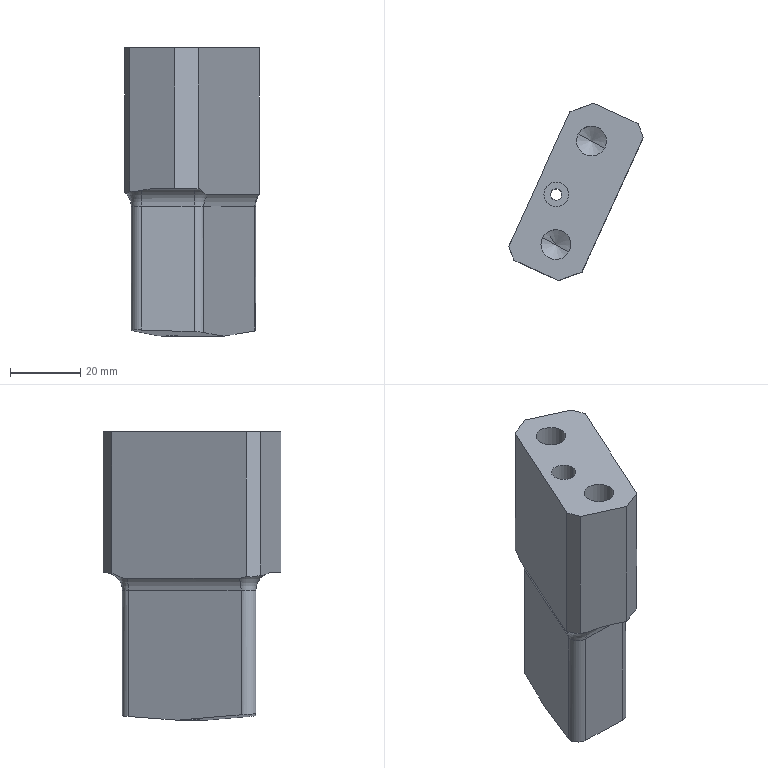Part | CATIA | 1 solid | 42 faces | box 38.266 x 50.474 x 82 mm | volume 71988 mm3 | plane 18 | cylinder 16 | torus 4 | cone 4 | commonest cylinder face diameters 6 x4 8.5 x4 10 x4 3.2 x2 7 x2
STEP:
#1=CARTESIAN_POINT('',(301.231,-29.493,29.));
#2=VERTEX_POINT('',#1);
#3=CARTESIAN_POINT('',(302.358,-29.072,28.988));
#4=VERTEX_POINT('',#3);
#5=CARTESIAN_POINT('',(302.358,-29.072,28.988));
#6=CARTESIAN_POINT('',(301.986,-29.211,28.994));
#7=CARTESIAN_POINT('',(301.611,-29.351,29.));
#8=CARTESIAN_POINT('',(301.231,-29.493,29.));
#9=B_SPLINE_CURVE_WITH_KNOTS('',3,(#5,#6,#7,#8),.UNSPECIFIED.,.F.,.U.,(4,4),(0.,1.722),.UNSPECIFIED.);
#10=EDGE_CURVE('',#2,#4,#9,.F.);
#11=ORIENTED_EDGE('',*,*,#10,.T.);
#12=CARTESIAN_POINT('',(302.358,-29.072,69.));
#13=VERTEX_POINT('',#12);
#14=CARTESIAN_POINT('',(302.358,-29.072,49.));
#15=DIRECTION('',(0.,0.,-1.));
#16=VECTOR('',#15,1.);
#17=LINE('',#14,#16);
#18=EDGE_CURVE('',#4,#13,#17,.F.);
#19=ORIENTED_EDGE('',*,*,#18,.T.);
#20=CARTESIAN_POINT('',(295.735,-31.548,69.));
#21=VERTEX_POINT('',#20);
#22=CARTESIAN_POINT('',(299.046,-30.31,69.));
#23=DIRECTION('',(0.9367,0.3502,0.));
#24=VECTOR('',#23,1.);
#25=LINE('',#22,#24);
#26=EDGE_CURVE('',#13,#21,#25,.F.);
#27=ORIENTED_EDGE('',*,*,#26,.T.);
#28=CARTESIAN_POINT('',(295.735,-31.548,29.));
#29=VERTEX_POINT('',#28);
#30=CARTESIAN_POINT('',(295.735,-31.548,49.));
#31=DIRECTION('',(0.,0.,-1.));
#32=VECTOR('',#31,1.);
#33=LINE('',#30,#32);
#34=EDGE_CURVE('',#21,#29,#33,.T.);
#35=ORIENTED_EDGE('',*,*,#34,.T.);
#36=CARTESIAN_POINT('',(301.212,-29.5,29.));
#37=VERTEX_POINT('',#36);
#38=CARTESIAN_POINT('',(299.046,-30.31,29.));
#39=DIRECTION('',(0.9367,0.3502,0.));
#40=VECTOR('',#39,1.);
#41=LINE('',#38,#40);
#42=EDGE_CURVE('',#29,#37,#41,.T.);
#43=ORIENTED_EDGE('',*,*,#42,.T.);
#44=CARTESIAN_POINT('',(301.231,-29.493,29.));
#45=CARTESIAN_POINT('',(301.224,-29.495,29.));
#46=CARTESIAN_POINT('',(301.218,-29.498,29.));
#47=CARTESIAN_POINT('',(301.212,-29.5,29.));
#48=B_SPLINE_CURVE_WITH_KNOTS('',3,(#44,#45,#46,#47),.UNSPECIFIED.,.F.,.U.,(4,4),(0.,0.02815),.UNSPECIFIED.);
#49=EDGE_CURVE('',#37,#2,#48,.F.);
#50=ORIENTED_EDGE('',*,*,#49,.T.);
#51=EDGE_LOOP('',(#11,#19,#27,#35,#43,#50));
#52=FACE_OUTER_BOUND('',#51,.T.);
#53=CARTESIAN_POINT('',(295.735,-31.548,77.));
#54=DIRECTION('',(0.3502,-0.9367,0.));
#55=DIRECTION('',(0.,0.,-1.));
#56=AXIS2_PLACEMENT_3D('',#53,#54,#55);
#57=PLANE('',#56);
#58=ADVANCED_FACE('',(#52),#57,.T.);
#59=ORIENTED_EDGE('',*,*,#18,.F.);
#60=CARTESIAN_POINT('',(305.025,-23.219,27.209));
#61=VERTEX_POINT('',#60);
#62=CARTESIAN_POINT('',(305.025,-23.219,27.209));
#63=CARTESIAN_POINT('',(304.904,-23.484,27.208));
#64=CARTESIAN_POINT('',(304.784,-23.749,27.238));
#65=CARTESIAN_POINT('',(304.662,-24.015,27.298));
#66=CARTESIAN_POINT('',(304.4,-24.59,27.479));
#67=CARTESIAN_POINT('',(304.124,-25.196,27.746));
#68=CARTESIAN_POINT('',(303.972,-25.53,27.902));
#69=CARTESIAN_POINT('',(303.682,-26.167,28.2));
#70=CARTESIAN_POINT('',(303.364,-26.864,28.484));
#71=CARTESIAN_POINT('',(303.214,-27.192,28.605));
#72=CARTESIAN_POINT('',(302.958,-27.756,28.782));
#73=CARTESIAN_POINT('',(302.688,-28.348,28.906));
#74=CARTESIAN_POINT('',(302.579,-28.587,28.945));
#75=CARTESIAN_POINT('',(302.469,-28.828,28.973));
#76=CARTESIAN_POINT('',(302.358,-29.072,28.988));
#77=B_SPLINE_CURVE_WITH_KNOTS('',5,(#62,#63,#64,#65,#66,#67,#68,#69,#70,#71,#72,#73,#74,#75,#76),.UNSPECIFIED.,.F.,.U.,(6,3,3,3,6),(0.,3.151,6.688,9.612,11.521),.UNSPECIFIED.);
#78=EDGE_CURVE('',#4,#61,#77,.F.);
#79=ORIENTED_EDGE('',*,*,#78,.T.);
#80=CARTESIAN_POINT('',(319.594,8.749,27.301));
#81=VERTEX_POINT('',#80);
#82=CARTESIAN_POINT('',(319.594,8.749,27.301));
#83=CARTESIAN_POINT('',(316.68,2.355,27.283));
#84=CARTESIAN_POINT('',(313.766,-4.038,27.265));
#85=CARTESIAN_POINT('',(310.852,-10.432,27.246));
#86=CARTESIAN_POINT('',(307.939,-16.826,27.228));
#87=CARTESIAN_POINT('',(305.025,-23.219,27.209));
#88=B_SPLINE_CURVE_WITH_KNOTS('',5,(#82,#83,#84,#85,#86,#87),.UNSPECIFIED.,.F.,.U.,(6,6),(0.,49.683),.UNSPECIFIED.);
#89=EDGE_CURVE('',#61,#81,#88,.F.);
#90=ORIENTED_EDGE('',*,*,#89,.T.);
#91=CARTESIAN_POINT('',(319.775,9.147,27.327));
#92=VERTEX_POINT('',#91);
#93=CARTESIAN_POINT('',(319.775,9.147,27.327));
#94=CARTESIAN_POINT('',(319.739,9.067,27.317));
#95=CARTESIAN_POINT('',(319.702,8.987,27.309));
#96=CARTESIAN_POINT('',(319.666,8.908,27.304));
#97=CARTESIAN_POINT('',(319.63,8.828,27.301));
#98=CARTESIAN_POINT('',(319.594,8.749,27.301));
#99=B_SPLINE_CURVE_WITH_KNOTS('',5,(#93,#94,#95,#96,#97,#98),.UNSPECIFIED.,.F.,.U.,(6,6),(0.,0.9322),.UNSPECIFIED.);
#100=EDGE_CURVE('',#81,#92,#99,.F.);
#101=ORIENTED_EDGE('',*,*,#100,.T.);
#102=CARTESIAN_POINT('',(319.775,9.147,69.));
#103=VERTEX_POINT('',#102);
#104=CARTESIAN_POINT('',(319.775,9.147,48.164));
#105=DIRECTION('',(0.,0.,1.));
#106=VECTOR('',#105,1.);
#107=LINE('',#104,#106);
#108=EDGE_CURVE('',#92,#103,#107,.T.);
#109=ORIENTED_EDGE('',*,*,#108,.T.);
#110=CARTESIAN_POINT('',(311.067,-9.962,69.));
#111=DIRECTION('',(0.4147,0.91,0.));
#112=VECTOR('',#111,1.);
#113=LINE('',#110,#112);
#114=EDGE_CURVE('',#103,#13,#113,.F.);
#115=ORIENTED_EDGE('',*,*,#114,.T.);
#116=EDGE_LOOP('',(#59,#79,#90,#101,#109,#115));
#117=FACE_OUTER_BOUND('',#116,.T.);
#118=CARTESIAN_POINT('',(300.284,-33.621,69.));
#119=DIRECTION('',(-0.91,0.4147,0.));
#120=DIRECTION('',(0.4147,0.91,0.));
#121=AXIS2_PLACEMENT_3D('',#118,#119,#120);
#122=PLANE('',#121);
#123=ADVANCED_FACE('',(#117),#122,.F.);
#124=CARTESIAN_POINT('',(318.289,13.121,26.491));
#125=VERTEX_POINT('',#124);
#126=CARTESIAN_POINT('',(318.289,13.121,69.));
#127=VERTEX_POINT('',#126);
#128=CARTESIAN_POINT('',(318.289,13.121,49.));
#129=DIRECTION('',(0.,0.,-1.));
#130=VECTOR('',#129,1.);
#131=LINE('',#128,#130);
#132=EDGE_CURVE('',#125,#127,#131,.F.);
#133=ORIENTED_EDGE('',*,*,#132,.T.);
#134=CARTESIAN_POINT('',(319.032,11.134,69.));
#135=DIRECTION('',(-0.3502,0.9367,0.));
#136=VECTOR('',#135,1.);
#137=LINE('',#134,#136);
#138=EDGE_CURVE('',#127,#103,#137,.F.);
#139=ORIENTED_EDGE('',*,*,#138,.T.);
#140=ORIENTED_EDGE('',*,*,#108,.F.);
#141=CARTESIAN_POINT('',(318.289,13.121,26.491));
#142=CARTESIAN_POINT('',(318.357,12.939,26.348));
#143=CARTESIAN_POINT('',(318.423,12.763,26.213));
#144=CARTESIAN_POINT('',(318.488,12.589,26.089));
#145=CARTESIAN_POINT('',(318.634,12.198,25.847));
#146=CARTESIAN_POINT('',(318.78,11.808,25.73));
#147=CARTESIAN_POINT('',(318.863,11.588,25.722));
#148=CARTESIAN_POINT('',(319.084,10.996,25.862));
#149=CARTESIAN_POINT('',(319.304,10.406,26.31));
#150=CARTESIAN_POINT('',(319.448,10.023,26.634));
#151=CARTESIAN_POINT('',(319.603,9.606,26.981));
#152=CARTESIAN_POINT('',(319.775,9.147,27.327));
#153=B_SPLINE_CURVE_WITH_KNOTS('',5,(#141,#142,#143,#144,#145,#146,#147,#148,#149,#150,#151,#152),.UNSPECIFIED.,.F.,.U.,(6,3,3,6),(0.,2.408,5.461,10.673),.UNSPECIFIED.);
#154=EDGE_CURVE('',#92,#125,#153,.F.);
#155=ORIENTED_EDGE('',*,*,#154,.T.);
#156=EDGE_LOOP('',(#133,#139,#140,#155));
#157=FACE_OUTER_BOUND('',#156,.T.);
#158=CARTESIAN_POINT('',(319.775,9.147,77.));
#159=DIRECTION('',(0.9367,0.3502,0.));
#160=DIRECTION('',(0.,0.,-1.));
#161=AXIS2_PLACEMENT_3D('',#158,#159,#160);
#162=PLANE('',#161);
#163=ADVANCED_FACE('',(#157),#162,.T.);
#164=CARTESIAN_POINT('',(305.55,18.927,29.));
#165=VERTEX_POINT('',#164);
#166=CARTESIAN_POINT('',(306.486,18.5,29.));
#167=VERTEX_POINT('',#166);
#168=CARTESIAN_POINT('',(306.018,18.713,29.));
#169=DIRECTION('',(0.91,-0.4147,0.));
#170=VECTOR('',#169,1.);
#171=LINE('',#168,#170);
#172=EDGE_CURVE('',#165,#167,#171,.T.);
#173=ORIENTED_EDGE('',*,*,#172,.F.);
#174=CARTESIAN_POINT('',(305.55,18.927,69.));
#175=VERTEX_POINT('',#174);
#176=CARTESIAN_POINT('',(305.55,18.927,49.));
#177=DIRECTION('',(0.,0.,-1.));
#178=VECTOR('',#177,1.);
#179=LINE('',#176,#178);
#180=EDGE_CURVE('',#175,#165,#179,.T.);
#181=ORIENTED_EDGE('',*,*,#180,.F.);
#182=CARTESIAN_POINT('',(311.92,16.024,69.));
#183=DIRECTION('',(0.91,-0.4147,0.));
#184=VECTOR('',#183,1.);
#185=LINE('',#182,#184);
#186=EDGE_CURVE('',#175,#127,#185,.T.);
#187=ORIENTED_EDGE('',*,*,#186,.T.);
#188=ORIENTED_EDGE('',*,*,#132,.F.);
#189=CARTESIAN_POINT('',(315.728,14.288,26.695));
#190=VERTEX_POINT('',#189);
#191=CARTESIAN_POINT('',(315.728,14.288,26.695));
#192=CARTESIAN_POINT('',(315.905,14.208,26.568));
#193=CARTESIAN_POINT('',(316.078,14.129,26.451));
#194=CARTESIAN_POINT('',(316.248,14.051,26.345));
#195=CARTESIAN_POINT('',(316.554,13.912,26.183));
#196=CARTESIAN_POINT('',(316.858,13.773,26.091));
#197=CARTESIAN_POINT('',(316.995,13.711,26.066));
#198=CARTESIAN_POINT('',(317.224,13.606,26.056));
#199=CARTESIAN_POINT('',(317.454,13.501,26.096));
#200=CARTESIAN_POINT('',(317.547,13.459,26.12));
#201=CARTESIAN_POINT('',(317.737,13.373,26.184));
#202=CARTESIAN_POINT('',(317.927,13.286,26.275));
#203=CARTESIAN_POINT('',(318.025,13.241,26.328));
#204=CARTESIAN_POINT('',(318.136,13.191,26.394));
#205=CARTESIAN_POINT('',(318.249,13.139,26.465));
#206=CARTESIAN_POINT('',(318.262,13.133,26.474));
#207=CARTESIAN_POINT('',(318.276,13.127,26.482));
#208=CARTESIAN_POINT('',(318.289,13.121,26.491));
#209=B_SPLINE_CURVE_WITH_KNOTS('',5,(#191,#192,#193,#194,#195,#196,#197,#198,#199,#200,#201,#202,#203,#204,#205,#206,#207,#208),.UNSPECIFIED.,.F.,.U.,(6,3,3,3,3,6),(0.,2.325,4.223,5.514,6.855,7.038),.UNSPECIFIED.);
#210=EDGE_CURVE('',#125,#190,#209,.F.);
#211=ORIENTED_EDGE('',*,*,#210,.T.);
#212=CARTESIAN_POINT('',(306.486,18.5,29.));
#213=CARTESIAN_POINT('',(307.081,18.229,29.));
#214=CARTESIAN_POINT('',(307.677,17.957,28.982));
#215=CARTESIAN_POINT('',(308.272,17.686,28.945));
#216=CARTESIAN_POINT('',(309.466,17.142,28.833));
#217=CARTESIAN_POINT('',(310.651,16.602,28.639));
#218=CARTESIAN_POINT('',(311.244,16.331,28.52));
#219=CARTESIAN_POINT('',(312.305,15.848,28.263));
#220=CARTESIAN_POINT('',(313.345,15.374,27.916));
#221=CARTESIAN_POINT('',(313.801,15.166,27.742));
#222=CARTESIAN_POINT('',(314.471,14.861,27.449));
#223=CARTESIAN_POINT('',(315.115,14.567,27.093));
#224=CARTESIAN_POINT('',(315.324,14.472,26.969));
#225=CARTESIAN_POINT('',(315.529,14.379,26.836));
#226=CARTESIAN_POINT('',(315.728,14.288,26.695));
#227=B_SPLINE_CURVE_WITH_KNOTS('',5,(#212,#213,#214,#215,#216,#217,#218,#219,#220,#221,#222,#223,#224,#225,#226),.UNSPECIFIED.,.F.,.U.,(6,3,3,3,6),(0.,4.628,9.309,13.064,14.907),.UNSPECIFIED.);
#228=EDGE_CURVE('',#190,#167,#227,.F.);
#229=ORIENTED_EDGE('',*,*,#228,.T.);
#230=EDGE_LOOP('',(#173,#181,#187,#188,#211,#229));
#231=FACE_OUTER_BOUND('',#230,.T.);
#232=CARTESIAN_POINT('',(301.,21.,69.));
#233=DIRECTION('',(0.4147,0.91,0.));
#234=DIRECTION('',(0.91,-0.4147,0.));
#235=AXIS2_PLACEMENT_3D('',#232,#233,#234);
#236=PLANE('',#235);
#237=ADVANCED_FACE('',(#231),#236,.T.);
#238=CARTESIAN_POINT('',(304.409,18.5,29.));
#239=VERTEX_POINT('',#238);
#240=CARTESIAN_POINT('',(300.859,17.173,28.821));
#241=VERTEX_POINT('',#240);
#242=CARTESIAN_POINT('',(304.409,18.5,29.));
#243=CARTESIAN_POINT('',(303.224,18.057,29.));
#244=CARTESIAN_POINT('',(302.039,17.614,28.942));
#245=CARTESIAN_POINT('',(300.859,17.173,28.821));
#246=B_SPLINE_CURVE_WITH_KNOTS('',3,(#242,#243,#244,#245),.UNSPECIFIED.,.F.,.U.,(4,4),(0.,5.368),.UNSPECIFIED.);
#247=EDGE_CURVE('',#239,#241,#246,.T.);
#248=ORIENTED_EDGE('',*,*,#247,.T.);
#249=CARTESIAN_POINT('',(298.927,16.45,28.686));
#250=VERTEX_POINT('',#249);
#251=CARTESIAN_POINT('',(300.859,17.173,28.821));
#252=CARTESIAN_POINT('',(300.196,16.925,28.752));
#253=CARTESIAN_POINT('',(299.559,16.687,28.697));
#254=CARTESIAN_POINT('',(298.927,16.45,28.686));
#255=B_SPLINE_CURVE_WITH_KNOTS('',3,(#251,#252,#253,#254),.UNSPECIFIED.,.F.,.U.,(4,4),(0.,3.29),.UNSPECIFIED.);
#256=EDGE_CURVE('',#241,#250,#255,.T.);
#257=ORIENTED_EDGE('',*,*,#256,.T.);
#258=CARTESIAN_POINT('',(298.927,16.45,69.));
#259=VERTEX_POINT('',#258);
#260=CARTESIAN_POINT('',(298.927,16.45,49.));
#261=DIRECTION('',(0.,0.,-1.));
#262=VECTOR('',#261,1.);
#263=LINE('',#260,#262);
#264=EDGE_CURVE('',#259,#250,#263,.T.);
#265=ORIENTED_EDGE('',*,*,#264,.F.);
#266=CARTESIAN_POINT('',(302.238,17.688,69.));
#267=DIRECTION('',(-0.9367,-0.3502,0.));
#268=VECTOR('',#267,1.);
#269=LINE('',#266,#268);
#270=EDGE_CURVE('',#259,#175,#269,.F.);
#271=ORIENTED_EDGE('',*,*,#270,.T.);
#272=ORIENTED_EDGE('',*,*,#180,.T.);
#273=CARTESIAN_POINT('',(302.238,17.688,29.));
#274=DIRECTION('',(-0.9367,-0.3502,0.));
#275=VECTOR('',#274,1.);
#276=LINE('',#273,#275);
#277=EDGE_CURVE('',#165,#239,#276,.T.);
#278=ORIENTED_EDGE('',*,*,#277,.T.);
#279=EDGE_LOOP('',(#248,#257,#265,#271,#272,#278));
#280=FACE_OUTER_BOUND('',#279,.T.);
#281=CARTESIAN_POINT('',(305.55,18.927,77.));
#282=DIRECTION('',(-0.3502,0.9367,0.));
#283=DIRECTION('',(0.,0.,-1.));
#284=AXIS2_PLACEMENT_3D('',#281,#282,#283);
#285=PLANE('',#284);
#286=ADVANCED_FACE('',(#280),#285,.T.);
#287=ORIENTED_EDGE('',*,*,#264,.T.);
#288=CARTESIAN_POINT('',(297.01,12.244,27.28));
#289=VERTEX_POINT('',#288);
#290=CARTESIAN_POINT('',(298.927,16.45,28.686));
#291=CARTESIAN_POINT('',(298.767,16.1,28.581));
#292=CARTESIAN_POINT('',(298.613,15.763,28.459));
#293=CARTESIAN_POINT('',(298.466,15.439,28.329));
#294=CARTESIAN_POINT('',(298.208,14.873,28.085));
#295=CARTESIAN_POINT('',(297.967,14.344,27.849));
#296=CARTESIAN_POINT('',(297.861,14.112,27.748));
#297=CARTESIAN_POINT('',(297.621,13.586,27.531));
#298=CARTESIAN_POINT('',(297.392,13.084,27.374));
#299=CARTESIAN_POINT('',(297.264,12.802,27.31));
#300=CARTESIAN_POINT('',(297.137,12.523,27.279));
#301=CARTESIAN_POINT('',(297.01,12.244,27.28));
#302=B_SPLINE_CURVE_WITH_KNOTS('',5,(#290,#291,#292,#293,#294,#295,#296,#297,#298,#299,#300,#301),.UNSPECIFIED.,.F.,.U.,(6,3,3,6),(0.,3.002,5.476,8.763),.UNSPECIFIED.);
#303=EDGE_CURVE('',#250,#289,#302,.T.);
#304=ORIENTED_EDGE('',*,*,#303,.T.);
#305=CARTESIAN_POINT('',(282.441,-19.724,27.368));
#306=VERTEX_POINT('',#305);
#307=CARTESIAN_POINT('',(297.01,12.244,27.28));
#308=CARTESIAN_POINT('',(294.096,5.85,27.298));
#309=CARTESIAN_POINT('',(291.182,-0.5432,27.315));
#310=CARTESIAN_POINT('',(288.268,-6.937,27.333));
#311=CARTESIAN_POINT('',(285.355,-13.33,27.35));
#312=CARTESIAN_POINT('',(282.441,-19.724,27.368));
#313=B_SPLINE_CURVE_WITH_KNOTS('',5,(#307,#308,#309,#310,#311,#312),.UNSPECIFIED.,.F.,.U.,(6,6),(0.,49.683),.UNSPECIFIED.);
#314=EDGE_CURVE('',#289,#306,#313,.T.);
#315=ORIENTED_EDGE('',*,*,#314,.T.);
#316=CARTESIAN_POINT('',(281.509,-21.768,27.891));
#317=VERTEX_POINT('',#316);
#318=CARTESIAN_POINT('',(282.441,-19.724,27.368));
#319=CARTESIAN_POINT('',(282.315,-20.,27.368));
#320=CARTESIAN_POINT('',(282.19,-20.275,27.398));
#321=CARTESIAN_POINT('',(282.063,-20.553,27.458));
#322=CARTESIAN_POINT('',(281.879,-20.958,27.577));
#323=CARTESIAN_POINT('',(281.687,-21.378,27.734));
#324=CARTESIAN_POINT('',(281.629,-21.506,27.784));
#325=CARTESIAN_POINT('',(281.57,-21.636,27.836));
#326=CARTESIAN_POINT('',(281.509,-21.768,27.891));
#327=B_SPLINE_CURVE_WITH_KNOTS('',5,(#318,#319,#320,#321,#322,#323,#324,#325,#326),.UNSPECIFIED.,.F.,.U.,(6,3,6),(0.,3.198,4.578),.UNSPECIFIED.);
#328=EDGE_CURVE('',#306,#317,#327,.T.);
#329=ORIENTED_EDGE('',*,*,#328,.T.);
#330=CARTESIAN_POINT('',(281.509,-21.768,69.));
#331=VERTEX_POINT('',#330);
#332=CARTESIAN_POINT('',(281.509,-21.768,48.445));
#333=DIRECTION('',(0.,0.,-1.));
#334=VECTOR('',#333,1.);
#335=LINE('',#332,#334);
#336=EDGE_CURVE('',#331,#317,#335,.T.);
#337=ORIENTED_EDGE('',*,*,#336,.F.);
#338=CARTESIAN_POINT('',(290.218,-2.659,69.));
#339=DIRECTION('',(-0.4147,-0.91,0.));
#340=VECTOR('',#339,1.);
#341=LINE('',#338,#340);
#342=EDGE_CURVE('',#331,#259,#341,.F.);
#343=ORIENTED_EDGE('',*,*,#342,.T.);
#344=EDGE_LOOP('',(#287,#304,#315,#329,#337,#343));
#345=FACE_OUTER_BOUND('',#344,.T.);
#346=CARTESIAN_POINT('',(301.,21.,69.));
#347=DIRECTION('',(0.91,-0.4147,0.));
#348=DIRECTION('',(-0.4147,-0.91,0.));
#349=AXIS2_PLACEMENT_3D('',#346,#347,#348);
#350=PLANE('',#349);
#351=ADVANCED_FACE('',(#345),#350,.F.);
#352=CARTESIAN_POINT('',(282.995,-25.742,69.));
#353=VERTEX_POINT('',#352);
#354=CARTESIAN_POINT('',(282.995,-25.742,28.28));
#355=VERTEX_POINT('',#354);
#356=CARTESIAN_POINT('',(282.995,-25.742,49.));
#357=DIRECTION('',(0.,0.,-1.));
#358=VECTOR('',#357,1.);
#359=LINE('',#356,#358);
#360=EDGE_CURVE('',#353,#355,#359,.T.);
#361=ORIENTED_EDGE('',*,*,#360,.F.);
#362=CARTESIAN_POINT('',(282.252,-23.755,69.));
#363=DIRECTION('',(0.3502,-0.9367,0.));
#364=VECTOR('',#363,1.);
#365=LINE('',#362,#364);
#366=EDGE_CURVE('',#353,#331,#365,.F.);
#367=ORIENTED_EDGE('',*,*,#366,.T.);
#368=ORIENTED_EDGE('',*,*,#336,.T.);
#369=CARTESIAN_POINT('',(281.509,-21.768,27.891));
#370=CARTESIAN_POINT('',(281.808,-22.567,27.686));
#371=CARTESIAN_POINT('',(282.09,-23.321,27.591));
#372=CARTESIAN_POINT('',(282.371,-24.073,27.72));
#373=CARTESIAN_POINT('',(282.668,-24.867,27.989));
#374=CARTESIAN_POINT('',(282.995,-25.742,28.28));
#375=B_SPLINE_CURVE_WITH_KNOTS('',5,(#369,#370,#371,#372,#373,#374),.UNSPECIFIED.,.F.,.U.,(6,6),(0.,8.172),.UNSPECIFIED.);
#376=EDGE_CURVE('',#317,#355,#375,.T.);
#377=ORIENTED_EDGE('',*,*,#376,.T.);
#378=EDGE_LOOP('',(#361,#367,#368,#377));
#379=FACE_OUTER_BOUND('',#378,.T.);
#380=CARTESIAN_POINT('',(281.509,-21.768,77.));
#381=DIRECTION('',(-0.9367,-0.3502,0.));
#382=DIRECTION('',(0.,0.,-1.));
#383=AXIS2_PLACEMENT_3D('',#380,#381,#382);
#384=PLANE('',#383);
#385=ADVANCED_FACE('',(#379),#384,.T.);
#386=CARTESIAN_POINT('',(291.241,-29.5,29.));
#387=VERTEX_POINT('',#386);
#388=CARTESIAN_POINT('',(293.488,-30.524,29.));
#389=DIRECTION('',(-0.91,0.4147,0.));
#390=VECTOR('',#389,1.);
#391=LINE('',#388,#390);
#392=EDGE_CURVE('',#29,#387,#391,.T.);
#393=ORIENTED_EDGE('',*,*,#392,.F.);
#394=ORIENTED_EDGE('',*,*,#34,.F.);
#395=CARTESIAN_POINT('',(289.365,-28.645,69.));
#396=DIRECTION('',(-0.91,0.4147,0.));
#397=VECTOR('',#396,1.);
#398=LINE('',#395,#397);
#399=EDGE_CURVE('',#21,#353,#398,.T.);
#400=ORIENTED_EDGE('',*,*,#399,.T.);
#401=ORIENTED_EDGE('',*,*,#360,.T.);
#402=CARTESIAN_POINT('',(286.362,-27.276,28.478));
#403=VERTEX_POINT('',#402);
#404=CARTESIAN_POINT('',(282.995,-25.742,28.28));
#405=CARTESIAN_POINT('',(283.359,-25.908,28.222));
#406=CARTESIAN_POINT('',(283.716,-26.071,28.182));
#407=CARTESIAN_POINT('',(284.069,-26.232,28.166));
#408=CARTESIAN_POINT('',(284.727,-26.532,28.183));
#409=CARTESIAN_POINT('',(285.397,-26.837,28.277));
#410=CARTESIAN_POINT('',(285.711,-26.98,28.335));
#411=CARTESIAN_POINT('',(286.032,-27.126,28.404));
#412=CARTESIAN_POINT('',(286.362,-27.276,28.478));
#413=B_SPLINE_CURVE_WITH_KNOTS('',5,(#404,#405,#406,#407,#408,#409,#410,#411,#412),.UNSPECIFIED.,.F.,.U.,(6,3,6),(0.,3.551,6.604),.UNSPECIFIED.);
#414=EDGE_CURVE('',#355,#403,#413,.T.);
#415=ORIENTED_EDGE('',*,*,#414,.T.);
#416=CARTESIAN_POINT('',(286.362,-27.276,28.478));
#417=CARTESIAN_POINT('',(286.953,-27.546,28.612));
#418=CARTESIAN_POINT('',(287.55,-27.818,28.722));
#419=CARTESIAN_POINT('',(288.149,-28.091,28.81));
#420=CARTESIAN_POINT('',(289.126,-28.536,28.92));
#421=CARTESIAN_POINT('',(290.107,-28.983,28.978));
#422=CARTESIAN_POINT('',(290.485,-29.155,28.993));
#423=CARTESIAN_POINT('',(290.863,-29.328,29.));
#424=CARTESIAN_POINT('',(291.241,-29.5,29.));
#425=B_SPLINE_CURVE_WITH_KNOTS('',5,(#416,#417,#418,#419,#420,#421,#422,#423,#424),.UNSPECIFIED.,.F.,.U.,(6,3,6),(0.,4.695,7.632),.UNSPECIFIED.);
#426=EDGE_CURVE('',#403,#387,#425,.T.);
#427=ORIENTED_EDGE('',*,*,#426,.T.);
#428=EDGE_LOOP('',(#393,#394,#400,#401,#415,#427));
#429=FACE_OUTER_BOUND('',#428,.T.);
#430=CARTESIAN_POINT('',(300.284,-33.621,69.));
#431=DIRECTION('',(-0.4147,-0.91,0.));
#432=DIRECTION('',(-0.91,0.4147,0.));
#433=AXIS2_PLACEMENT_3D('',#430,#431,#432);
#434=PLANE('',#433);
#435=ADVANCED_FACE('',(#429),#434,.T.);
#436=ORIENTED_EDGE('',*,*,#42,.F.);
#437=ORIENTED_EDGE('',*,*,#392,.T.);
#438=CARTESIAN_POINT('',(296.226,-29.5,29.));
#439=DIRECTION('',(-1.,0.,0.));
#440=VECTOR('',#439,1.);
#441=LINE('',#438,#440);
#442=EDGE_CURVE('',#37,#387,#441,.T.);
#443=ORIENTED_EDGE('',*,*,#442,.F.);
#444=EDGE_LOOP('',(#436,#437,#443));
#445=FACE_OUTER_BOUND('',#444,.T.);
#446=CARTESIAN_POINT('',(0.,0.,29.));
#447=DIRECTION('',(0.,0.,-1.));
#448=DIRECTION('',(0.,1.,0.));
#449=AXIS2_PLACEMENT_3D('',#446,#447,#448);
#450=PLANE('',#449);
#451=ADVANCED_FACE('',(#445),#450,.T.);
#452=ORIENTED_EDGE('',*,*,#277,.F.);
#453=ORIENTED_EDGE('',*,*,#172,.T.);
#454=CARTESIAN_POINT('',(305.447,18.5,29.));
#455=DIRECTION('',(-1.,-0.000000028,0.));
#456=VECTOR('',#455,1.);
#457=LINE('',#454,#456);
#458=EDGE_CURVE('',#239,#167,#457,.F.);
#459=ORIENTED_EDGE('',*,*,#458,.F.);
#460=EDGE_LOOP('',(#452,#453,#459));
#461=FACE_OUTER_BOUND('',#460,.T.);
#462=ADVANCED_FACE('',(#461),#450,.T.);
#463=CARTESIAN_POINT('',(286.362,-24.5,24.));
#464=VERTEX_POINT('',#463);
#465=CARTESIAN_POINT('',(286.362,-29.5,24.));
#466=DIRECTION('',(-1.,0.,0.));
#467=AXIS2_PLACEMENT_3D('',#465,#466,$);
#468=CIRCLE('',#467,5.);
#469=EDGE_CURVE('',#403,#464,#468,.T.);
#470=ORIENTED_EDGE('',*,*,#469,.T.);
#471=CARTESIAN_POINT('',(301.231,-24.5,24.));
#472=VERTEX_POINT('',#471);
#473=CARTESIAN_POINT('',(302.262,-24.5,24.));
#474=DIRECTION('',(-1.,0.,0.));
#475=VECTOR('',#474,1.);
#476=LINE('',#473,#475);
#477=EDGE_CURVE('',#472,#464,#476,.T.);
#478=ORIENTED_EDGE('',*,*,#477,.F.);
#479=CARTESIAN_POINT('',(301.231,-29.5,24.));
#480=DIRECTION('',(-1.,0.,0.));
#481=AXIS2_PLACEMENT_3D('',#479,#480,$);
#482=CIRCLE('',#481,5.);
#483=EDGE_CURVE('',#2,#472,#482,.T.);
#484=ORIENTED_EDGE('',*,*,#483,.F.);
#485=ORIENTED_EDGE('',*,*,#49,.F.);
#486=ORIENTED_EDGE('',*,*,#442,.T.);
#487=ORIENTED_EDGE('',*,*,#426,.F.);
#488=EDGE_LOOP('',(#470,#478,#484,#485,#486,#487));
#489=FACE_OUTER_BOUND('',#488,.T.);
#490=CARTESIAN_POINT('',(302.262,-29.5,24.));
#491=DIRECTION('',(-1.,0.,0.));
#492=DIRECTION('',(0.,0.,1.));
#493=AXIS2_PLACEMENT_3D('',#490,#491,#492);
#494=CYLINDRICAL_SURFACE('',#493,5.);
#495=ADVANCED_FACE('',(#489),#494,.F.);
#496=CARTESIAN_POINT('',(283.629,-20.262,24.));
#497=VERTEX_POINT('',#496);
#498=CARTESIAN_POINT('',(279.075,-18.199,24.));
#499=DIRECTION('',(-0.4127,-0.9109,0.));
#500=AXIS2_PLACEMENT_3D('',#498,#499,$);
#501=CIRCLE('',#500,5.);
#502=EDGE_CURVE('',#306,#497,#501,.F.);
#503=ORIENTED_EDGE('',*,*,#502,.T.);
#504=CARTESIAN_POINT('',(286.362,-21.5,24.));
#505=DIRECTION('',(0.,0.,-1.));
#506=AXIS2_PLACEMENT_3D('',#504,#505,$);
#507=CIRCLE('',#506,3.);
#508=EDGE_CURVE('',#464,#497,#507,.T.);
#509=ORIENTED_EDGE('',*,*,#508,.F.);
#510=ORIENTED_EDGE('',*,*,#469,.F.);
#511=ORIENTED_EDGE('',*,*,#414,.F.);
#512=ORIENTED_EDGE('',*,*,#376,.F.);
#513=ORIENTED_EDGE('',*,*,#328,.F.);
#514=EDGE_LOOP('',(#503,#509,#510,#511,#512,#513));
#515=FACE_OUTER_BOUND('',#514,.T.);
#516=CARTESIAN_POINT('',(286.362,-21.5,24.));
#517=DIRECTION('',(0.,0.,-1.));
#518=DIRECTION('',(0.3102,-0.9507,0.));
#519=AXIS2_PLACEMENT_3D('',#516,#517,#518);
#520=TOROIDAL_SURFACE('',#519,8.,5.);
#521=ADVANCED_FACE('',(#515),#520,.F.);
#522=ORIENTED_EDGE('',*,*,#483,.T.);
#523=CARTESIAN_POINT('',(303.963,-22.738,24.));
#524=VERTEX_POINT('',#523);
#525=CARTESIAN_POINT('',(301.231,-21.5,24.));
#526=DIRECTION('',(0.,0.,-1.));
#527=AXIS2_PLACEMENT_3D('',#525,#526,$);
#528=CIRCLE('',#527,3.);
#529=EDGE_CURVE('',#524,#472,#528,.T.);
#530=ORIENTED_EDGE('',*,*,#529,.F.);
#531=CARTESIAN_POINT('',(308.518,-24.801,24.));
#532=DIRECTION('',(0.4127,0.9109,0.));
#533=AXIS2_PLACEMENT_3D('',#531,#532,$);
#534=CIRCLE('',#533,5.);
#535=EDGE_CURVE('',#61,#524,#534,.F.);
#536=ORIENTED_EDGE('',*,*,#535,.F.);
#537=ORIENTED_EDGE('',*,*,#78,.F.);
#538=ORIENTED_EDGE('',*,*,#10,.F.);
#539=EDGE_LOOP('',(#522,#530,#536,#537,#538));
#540=FACE_OUTER_BOUND('',#539,.T.);
#541=CARTESIAN_POINT('',(301.231,-21.5,24.));
#542=DIRECTION('',(0.,0.,-1.));
#543=DIRECTION('',(0.9995,-0.0318,0.));
#544=AXIS2_PLACEMENT_3D('',#541,#542,#543);
#545=TOROIDAL_SURFACE('',#544,8.,5.);
#546=ADVANCED_FACE('',(#540),#545,.F.);
#547=CARTESIAN_POINT('',(298.126,11.738,24.));
#548=VERTEX_POINT('',#547);
#549=CARTESIAN_POINT('',(293.572,13.801,24.));
#550=DIRECTION('',(-0.4127,-0.9109,0.));
#551=AXIS2_PLACEMENT_3D('',#549,#550,$);
#552=CIRCLE('',#551,5.);
#553=EDGE_CURVE('',#289,#548,#552,.F.);
#554=ORIENTED_EDGE('',*,*,#553,.T.);
#555=CARTESIAN_POINT('',(291.716,-2.411,24.));
#556=DIRECTION('',(-0.4127,-0.9109,0.));
#557=VECTOR('',#556,1.);
#558=LINE('',#555,#557);
#559=EDGE_CURVE('',#497,#548,#558,.F.);
#560=ORIENTED_EDGE('',*,*,#559,.F.);
#561=ORIENTED_EDGE('',*,*,#502,.F.);
#562=ORIENTED_EDGE('',*,*,#314,.F.);
#563=EDGE_LOOP('',(#554,#560,#561,#562));
#564=FACE_OUTER_BOUND('',#563,.T.);
#565=CARTESIAN_POINT('',(287.162,-0.348,24.));
#566=DIRECTION('',(-0.4127,-0.9109,0.));
#567=DIRECTION('',(0.9109,-0.4127,0.));
#568=AXIS2_PLACEMENT_3D('',#565,#566,#567);
#569=CYLINDRICAL_SURFACE('',#568,5.);
#570=ADVANCED_FACE('',(#564),#569,.F.);
#571=ORIENTED_EDGE('',*,*,#535,.T.);
#572=CARTESIAN_POINT('',(318.46,9.262,24.));
#573=VERTEX_POINT('',#572);
#574=CARTESIAN_POINT('',(311.547,-5.997,24.));
#575=DIRECTION('',(0.4127,0.9109,0.));
#576=VECTOR('',#575,1.);
#577=LINE('',#574,#576);
#578=EDGE_CURVE('',#573,#524,#577,.F.);
#579=ORIENTED_EDGE('',*,*,#578,.F.);
#580=CARTESIAN_POINT('',(323.015,7.199,24.));
#581=DIRECTION('',(0.4127,0.9109,0.));
#582=AXIS2_PLACEMENT_3D('',#580,#581,$);
#583=CIRCLE('',#582,5.);
#584=EDGE_CURVE('',#81,#573,#583,.F.);
#585=ORIENTED_EDGE('',*,*,#584,.F.);
#586=ORIENTED_EDGE('',*,*,#89,.F.);
#587=EDGE_LOOP('',(#571,#579,#585,#586));
#588=FACE_OUTER_BOUND('',#587,.T.);
#589=CARTESIAN_POINT('',(316.102,-8.06,24.));
#590=DIRECTION('',(0.4127,0.9109,0.));
#591=DIRECTION('',(-0.9109,0.4127,0.));
#592=AXIS2_PLACEMENT_3D('',#589,#590,#591);
#593=CYLINDRICAL_SURFACE('',#592,5.);
#594=ADVANCED_FACE('',(#588),#593,.F.);
#595=ORIENTED_EDGE('',*,*,#584,.T.);
#596=CARTESIAN_POINT('',(315.728,13.5,24.));
#597=VERTEX_POINT('',#596);
#598=CARTESIAN_POINT('',(315.728,10.5,24.));
#599=DIRECTION('',(0.,0.,-1.));
#600=AXIS2_PLACEMENT_3D('',#598,#599,$);
#601=CIRCLE('',#600,3.);
#602=EDGE_CURVE('',#597,#573,#601,.T.);
#603=ORIENTED_EDGE('',*,*,#602,.F.);
#604=CARTESIAN_POINT('',(315.728,18.5,24.));
#605=DIRECTION('',(-1.,-0.000000028,0.));
#606=AXIS2_PLACEMENT_3D('',#604,#605,$);
#607=CIRCLE('',#606,5.);
#608=EDGE_CURVE('',#190,#597,#607,.F.);
#609=ORIENTED_EDGE('',*,*,#608,.F.);
#610=ORIENTED_EDGE('',*,*,#210,.F.);
#611=ORIENTED_EDGE('',*,*,#154,.F.);
#612=ORIENTED_EDGE('',*,*,#100,.F.);
#613=EDGE_LOOP('',(#595,#603,#609,#610,#611,#612));
#614=FACE_OUTER_BOUND('',#613,.T.);
#615=CARTESIAN_POINT('',(315.728,10.5,24.));
#616=DIRECTION('',(0.,0.,-1.));
#617=DIRECTION('',(-0.1637,0.9865,0.));
#618=AXIS2_PLACEMENT_3D('',#615,#616,#617);
#619=TOROIDAL_SURFACE('',#618,8.,5.);
#620=ADVANCED_FACE('',(#614),#619,.F.);
#621=CARTESIAN_POINT('',(300.859,13.5,24.));
#622=VERTEX_POINT('',#621);
#623=CARTESIAN_POINT('',(300.859,18.5,24.));
#624=DIRECTION('',(-1.,-0.000000028,0.));
#625=AXIS2_PLACEMENT_3D('',#623,#624,$);
#626=CIRCLE('',#625,5.);
#627=EDGE_CURVE('',#241,#622,#626,.F.);
#628=ORIENTED_EDGE('',*,*,#627,.T.);
#629=CARTESIAN_POINT('',(300.859,10.5,24.));
#630=DIRECTION('',(0.,0.,-1.));
#631=AXIS2_PLACEMENT_3D('',#629,#630,$);
#632=CIRCLE('',#631,3.);
#633=EDGE_CURVE('',#548,#622,#632,.T.);
#634=ORIENTED_EDGE('',*,*,#633,.F.);
#635=ORIENTED_EDGE('',*,*,#553,.F.);
#636=ORIENTED_EDGE('',*,*,#303,.F.);
#637=ORIENTED_EDGE('',*,*,#256,.F.);
#638=EDGE_LOOP('',(#628,#634,#635,#636,#637));
#639=FACE_OUTER_BOUND('',#638,.T.);
#640=CARTESIAN_POINT('',(300.859,10.5,24.));
#641=DIRECTION('',(0.,0.,-1.));
#642=DIRECTION('',(-0.9995,0.0318,0.));
#643=AXIS2_PLACEMENT_3D('',#640,#641,#642);
#644=TOROIDAL_SURFACE('',#643,8.,5.);
#645=ADVANCED_FACE('',(#639),#644,.F.);
#646=ORIENTED_EDGE('',*,*,#608,.T.);
#647=CARTESIAN_POINT('',(300.642,13.5,24.));
#648=DIRECTION('',(-1.,-0.000000028,0.));
#649=VECTOR('',#648,1.);
#650=LINE('',#647,#649);
#651=EDGE_CURVE('',#622,#597,#650,.F.);
#652=ORIENTED_EDGE('',*,*,#651,.F.);
#653=ORIENTED_EDGE('',*,*,#627,.F.);
#654=ORIENTED_EDGE('',*,*,#247,.F.);
#655=ORIENTED_EDGE('',*,*,#458,.T.);
#656=ORIENTED_EDGE('',*,*,#228,.F.);
#657=EDGE_LOOP('',(#646,#652,#653,#654,#655,#656));
#658=FACE_OUTER_BOUND('',#657,.T.);
#659=CARTESIAN_POINT('',(300.642,18.5,24.));
#660=DIRECTION('',(-1.,-0.000000028,0.));
#661=DIRECTION('',(0.000000028,-1.,0.));
#662=AXIS2_PLACEMENT_3D('',#659,#660,#661);
#663=CYLINDRICAL_SURFACE('',#662,5.);
#664=ADVANCED_FACE('',(#658),#663,.F.);
#665=CARTESIAN_POINT('',(298.5,-7.,46.));
#666=VERTEX_POINT('',#665);
#667=CARTESIAN_POINT('',(291.5,-7.,46.));
#668=VERTEX_POINT('',#667);
#669=CARTESIAN_POINT('',(295.,-7.,46.));
#670=DIRECTION('',(0.,0.,-1.));
#671=AXIS2_PLACEMENT_3D('',#669,#670,$);
#672=CIRCLE('',#671,3.5);
#673=EDGE_CURVE('',#666,#668,#672,.T.);
#674=ORIENTED_EDGE('',*,*,#673,.F.);
#675=CARTESIAN_POINT('',(295.,-7.,46.));
#676=DIRECTION('',(0.,0.,-1.));
#677=AXIS2_PLACEMENT_3D('',#675,#676,$);
#678=CIRCLE('',#677,3.5);
#679=EDGE_CURVE('',#668,#666,#678,.T.);
#680=ORIENTED_EDGE('',*,*,#679,.F.);
#681=EDGE_LOOP('',(#674,#680));
#682=FACE_OUTER_BOUND('',#681,.T.);
#683=CARTESIAN_POINT('',(296.6,-7.,46.));
#684=VERTEX_POINT('',#683);
#685=CARTESIAN_POINT('',(293.4,-7.,46.));
#686=VERTEX_POINT('',#685);
#687=CARTESIAN_POINT('',(295.,-7.,46.));
#688=DIRECTION('',(0.,0.,-1.));
#689=AXIS2_PLACEMENT_3D('',#687,#688,$);
#690=CIRCLE('',#689,1.6);
#691=EDGE_CURVE('',#684,#686,#690,.T.);
#692=ORIENTED_EDGE('',*,*,#691,.T.);
#693=CARTESIAN_POINT('',(295.,-7.,46.));
#694=DIRECTION('',(0.,0.,-1.));
#695=AXIS2_PLACEMENT_3D('',#693,#694,$);
#696=CIRCLE('',#695,1.6);
#697=EDGE_CURVE('',#686,#684,#696,.T.);
#698=ORIENTED_EDGE('',*,*,#697,.T.);
#699=EDGE_LOOP('',(#692,#698));
#700=FACE_BOUND('',#699,.T.);
#701=CARTESIAN_POINT('',(295.,-7.,46.));
#702=DIRECTION('',(0.,0.,-1.));
#703=DIRECTION('',(-1.,0.,0.));
#704=AXIS2_PLACEMENT_3D('',#701,#702,#703);
#705=PLANE('',#704);
#706=ADVANCED_FACE('',(#682,#700),#705,.F.);
#707=ORIENTED_EDGE('',*,*,#679,.T.);
#708=CARTESIAN_POINT('',(298.5,-7.,69.));
#709=VERTEX_POINT('',#708);
#710=CARTESIAN_POINT('',(298.5,-7.,57.5));
#711=DIRECTION('',(0.,0.,-1.));
#712=VECTOR('',#711,1.);
#713=LINE('',#710,#712);
#714=EDGE_CURVE('',#709,#666,#713,.T.);
#715=ORIENTED_EDGE('',*,*,#714,.F.);
#716=CARTESIAN_POINT('',(291.5,-7.,69.));
#717=VERTEX_POINT('',#716);
#718=CARTESIAN_POINT('',(295.,-7.,69.));
#719=DIRECTION('',(0.,0.,-1.));
#720=AXIS2_PLACEMENT_3D('',#718,#719,$);
#721=CIRCLE('',#720,3.5);
#722=EDGE_CURVE('',#717,#709,#721,.T.);
#723=ORIENTED_EDGE('',*,*,#722,.F.);
#724=CARTESIAN_POINT('',(291.5,-7.,57.5));
#725=DIRECTION('',(0.,0.,-1.));
#726=VECTOR('',#725,1.);
#727=LINE('',#724,#726);
#728=EDGE_CURVE('',#717,#668,#727,.T.);
#729=ORIENTED_EDGE('',*,*,#728,.T.);
#730=EDGE_LOOP('',(#707,#715,#723,#729));
#731=FACE_OUTER_BOUND('',#730,.T.);
#732=CARTESIAN_POINT('',(295.,-7.,57.5));
#733=DIRECTION('',(0.,0.,-1.));
#734=DIRECTION('',(-1.,0.,0.));
#735=AXIS2_PLACEMENT_3D('',#732,#733,#734);
#736=CYLINDRICAL_SURFACE('',#735,3.5);
#737=ADVANCED_FACE('',(#731),#736,.F.);
#738=ORIENTED_EDGE('',*,*,#673,.T.);
#739=ORIENTED_EDGE('',*,*,#728,.F.);
#740=CARTESIAN_POINT('',(295.,-7.,69.));
#741=DIRECTION('',(0.,0.,-1.));
#742=AXIS2_PLACEMENT_3D('',#740,#741,$);
#743=CIRCLE('',#742,3.5);
#744=EDGE_CURVE('',#709,#717,#743,.T.);
#745=ORIENTED_EDGE('',*,*,#744,.F.);
#746=ORIENTED_EDGE('',*,*,#714,.T.);
#747=EDGE_LOOP('',(#738,#739,#745,#746));
#748=FACE_OUTER_BOUND('',#747,.T.);
#749=ADVANCED_FACE('',(#748),#736,.F.);
#750=ORIENTED_EDGE('',*,*,#186,.F.);
#751=ORIENTED_EDGE('',*,*,#270,.F.);
#752=ORIENTED_EDGE('',*,*,#342,.F.);
#753=ORIENTED_EDGE('',*,*,#366,.F.);
#754=ORIENTED_EDGE('',*,*,#399,.F.);
#755=ORIENTED_EDGE('',*,*,#26,.F.);
#756=ORIENTED_EDGE('',*,*,#114,.F.);
#757=ORIENTED_EDGE('',*,*,#138,.F.);
#758=EDGE_LOOP('',(#750,#751,#752,#753,#754,#755,#756,#757));
#759=FACE_OUTER_BOUND('',#758,.T.);
#760=ORIENTED_EDGE('',*,*,#722,.T.);
#761=ORIENTED_EDGE('',*,*,#744,.T.);
#762=EDGE_LOOP('',(#760,#761));
#763=FACE_BOUND('',#762,.T.);
#764=CARTESIAN_POINT('',(298.647,-23.322,69.));
#765=VERTEX_POINT('',#764);
#766=CARTESIAN_POINT('',(291.187,-19.247,69.));
#767=VERTEX_POINT('',#766);
#768=CARTESIAN_POINT('',(294.917,-21.285,69.));
#769=DIRECTION('',(0.,0.,1.));
#770=AXIS2_PLACEMENT_3D('',#768,#769,$);
#771=CIRCLE('',#770,4.25);
#772=EDGE_CURVE('',#765,#767,#771,.T.);
#773=ORIENTED_EDGE('',*,*,#772,.F.);
#774=CARTESIAN_POINT('',(294.917,-21.285,69.));
#775=DIRECTION('',(0.,0.,1.));
#776=AXIS2_PLACEMENT_3D('',#774,#775,$);
#777=CIRCLE('',#776,4.25);
#778=EDGE_CURVE('',#767,#765,#777,.T.);
#779=ORIENTED_EDGE('',*,*,#778,.F.);
#780=EDGE_LOOP('',(#773,#779));
#781=FACE_BOUND('',#780,.T.);
#782=CARTESIAN_POINT('',(308.772,6.131,69.));
#783=VERTEX_POINT('',#782);
#784=CARTESIAN_POINT('',(301.313,10.206,69.));
#785=VERTEX_POINT('',#784);
#786=CARTESIAN_POINT('',(305.043,8.168,69.));
#787=DIRECTION('',(0.,0.,1.));
#788=AXIS2_PLACEMENT_3D('',#786,#787,$);
#789=CIRCLE('',#788,4.25);
#790=EDGE_CURVE('',#783,#785,#789,.T.);
#791=ORIENTED_EDGE('',*,*,#790,.F.);
#792=CARTESIAN_POINT('',(305.043,8.168,69.));
#793=DIRECTION('',(0.,0.,1.));
#794=AXIS2_PLACEMENT_3D('',#792,#793,$);
#795=CIRCLE('',#794,4.25);
#796=EDGE_CURVE('',#785,#783,#795,.T.);
#797=ORIENTED_EDGE('',*,*,#796,.F.);
#798=EDGE_LOOP('',(#791,#797));
#799=FACE_BOUND('',#798,.T.);
#800=CARTESIAN_POINT('',(0.,0.,69.));
#801=DIRECTION('',(0.,0.,1.));
#802=DIRECTION('',(1.,0.,0.));
#803=AXIS2_PLACEMENT_3D('',#800,#801,#802);
#804=PLANE('',#803);
#805=ADVANCED_FACE('',(#759,#763,#781,#799),#804,.T.);
#806=CARTESIAN_POINT('',(305.043,8.168,41.546));
#807=VERTEX_POINT('',#806);
#808=CARTESIAN_POINT('',(301.313,10.206,44.));
#809=VERTEX_POINT('',#808);
#810=CARTESIAN_POINT('',(303.178,9.187,42.773));
#811=DIRECTION('',(-0.76,0.4152,0.5));
#812=VECTOR('',#811,1.);
#813=LINE('',#810,#812);
#814=EDGE_CURVE('',#807,#809,#813,.T.);
#815=ORIENTED_EDGE('',*,*,#814,.T.);
#816=CARTESIAN_POINT('',(308.772,6.131,44.));
#817=VERTEX_POINT('',#816);
#818=CARTESIAN_POINT('',(305.043,8.168,44.));
#819=DIRECTION('',(0.,0.,1.));
#820=AXIS2_PLACEMENT_3D('',#818,#819,$);
#821=CIRCLE('',#820,4.25);
#822=EDGE_CURVE('',#817,#809,#821,.F.);
#823=ORIENTED_EDGE('',*,*,#822,.F.);
#824=CARTESIAN_POINT('',(306.908,7.149,42.773));
#825=DIRECTION('',(0.76,-0.4152,0.5));
#826=VECTOR('',#825,1.);
#827=LINE('',#824,#826);
#828=EDGE_CURVE('',#807,#817,#827,.T.);
#829=ORIENTED_EDGE('',*,*,#828,.F.);
#830=EDGE_LOOP('',(#815,#823,#829));
#831=FACE_OUTER_BOUND('',#830,.T.);
#832=CARTESIAN_POINT('',(305.043,8.168,41.546));
#833=DIRECTION('',(0.,0.,1.));
#834=DIRECTION('',(0.8776,-0.4794,0.));
#835=AXIS2_PLACEMENT_3D('',#832,#833,#834);
#836=CONICAL_SURFACE('',#835,0.,1.047);
#837=ADVANCED_FACE('',(#831),#836,.F.);
#838=ORIENTED_EDGE('',*,*,#828,.T.);
#839=CARTESIAN_POINT('',(305.043,8.168,44.));
#840=DIRECTION('',(0.,0.,1.));
#841=AXIS2_PLACEMENT_3D('',#839,#840,$);
#842=CIRCLE('',#841,4.25);
#843=EDGE_CURVE('',#809,#817,#842,.F.);
#844=ORIENTED_EDGE('',*,*,#843,.F.);
#845=ORIENTED_EDGE('',*,*,#814,.F.);
#846=EDGE_LOOP('',(#838,#844,#845));
#847=FACE_OUTER_BOUND('',#846,.T.);
#848=ADVANCED_FACE('',(#847),#836,.F.);
#849=ORIENTED_EDGE('',*,*,#796,.T.);
#850=CARTESIAN_POINT('',(308.772,6.131,56.655));
#851=DIRECTION('',(0.,0.,-1.));
#852=VECTOR('',#851,1.);
#853=LINE('',#850,#852);
#854=EDGE_CURVE('',#817,#783,#853,.F.);
#855=ORIENTED_EDGE('',*,*,#854,.F.);
#856=ORIENTED_EDGE('',*,*,#822,.T.);
#857=CARTESIAN_POINT('',(301.313,10.206,56.655));
#858=DIRECTION('',(0.,0.,-1.));
#859=VECTOR('',#858,1.);
#860=LINE('',#857,#859);
#861=EDGE_CURVE('',#809,#785,#860,.F.);
#862=ORIENTED_EDGE('',*,*,#861,.T.);
#863=EDGE_LOOP('',(#849,#855,#856,#862));
#864=FACE_OUTER_BOUND('',#863,.T.);
#865=CARTESIAN_POINT('',(305.043,8.168,68.9));
#866=DIRECTION('',(0.,0.,-1.));
#867=DIRECTION('',(0.8776,-0.4794,0.));
#868=AXIS2_PLACEMENT_3D('',#865,#866,#867);
#869=CYLINDRICAL_SURFACE('',#868,4.25);
#870=ADVANCED_FACE('',(#864),#869,.F.);
#871=ORIENTED_EDGE('',*,*,#790,.T.);
#872=ORIENTED_EDGE('',*,*,#861,.F.);
#873=ORIENTED_EDGE('',*,*,#843,.T.);
#874=ORIENTED_EDGE('',*,*,#854,.T.);
#875=EDGE_LOOP('',(#871,#872,#873,#874));
#876=FACE_OUTER_BOUND('',#875,.T.);
#877=ADVANCED_FACE('',(#876),#869,.F.);
#878=CARTESIAN_POINT('',(294.917,-21.285,41.546));
#879=VERTEX_POINT('',#878);
#880=CARTESIAN_POINT('',(291.187,-19.247,44.));
#881=VERTEX_POINT('',#880);
#882=CARTESIAN_POINT('',(293.052,-20.266,42.773));
#883=DIRECTION('',(-0.76,0.4152,0.5));
#884=VECTOR('',#883,1.);
#885=LINE('',#882,#884);
#886=EDGE_CURVE('',#879,#881,#885,.T.);
#887=ORIENTED_EDGE('',*,*,#886,.T.);
#888=CARTESIAN_POINT('',(298.647,-23.322,44.));
#889=VERTEX_POINT('',#888);
#890=CARTESIAN_POINT('',(294.917,-21.285,44.));
#891=DIRECTION('',(0.,0.,1.));
#892=AXIS2_PLACEMENT_3D('',#890,#891,$);
#893=CIRCLE('',#892,4.25);
#894=EDGE_CURVE('',#889,#881,#893,.F.);
#895=ORIENTED_EDGE('',*,*,#894,.F.);
#896=CARTESIAN_POINT('',(296.782,-22.304,42.773));
#897=DIRECTION('',(0.76,-0.4152,0.5));
#898=VECTOR('',#897,1.);
#899=LINE('',#896,#898);
#900=EDGE_CURVE('',#879,#889,#899,.T.);
#901=ORIENTED_EDGE('',*,*,#900,.F.);
#902=EDGE_LOOP('',(#887,#895,#901));
#903=FACE_OUTER_BOUND('',#902,.T.);
#904=CARTESIAN_POINT('',(294.917,-21.285,41.546));
#905=DIRECTION('',(0.,0.,1.));
#906=DIRECTION('',(0.8776,-0.4794,0.));
#907=AXIS2_PLACEMENT_3D('',#904,#905,#906);
#908=CONICAL_SURFACE('',#907,0.,1.047);
#909=ADVANCED_FACE('',(#903),#908,.F.);
#910=ORIENTED_EDGE('',*,*,#900,.T.);
#911=CARTESIAN_POINT('',(294.917,-21.285,44.));
#912=DIRECTION('',(0.,0.,1.));
#913=AXIS2_PLACEMENT_3D('',#911,#912,$);
#914=CIRCLE('',#913,4.25);
#915=EDGE_CURVE('',#881,#889,#914,.F.);
#916=ORIENTED_EDGE('',*,*,#915,.F.);
#917=ORIENTED_EDGE('',*,*,#886,.F.);
#918=EDGE_LOOP('',(#910,#916,#917));
#919=FACE_OUTER_BOUND('',#918,.T.);
#920=ADVANCED_FACE('',(#919),#908,.F.);
#921=ORIENTED_EDGE('',*,*,#778,.T.);
#922=CARTESIAN_POINT('',(298.647,-23.322,56.655));
#923=DIRECTION('',(0.,0.,-1.));
#924=VECTOR('',#923,1.);
#925=LINE('',#922,#924);
#926=EDGE_CURVE('',#889,#765,#925,.F.);
#927=ORIENTED_EDGE('',*,*,#926,.F.);
#928=ORIENTED_EDGE('',*,*,#894,.T.);
#929=CARTESIAN_POINT('',(291.187,-19.247,56.655));
#930=DIRECTION('',(0.,0.,-1.));
#931=VECTOR('',#930,1.);
#932=LINE('',#929,#931);
#933=EDGE_CURVE('',#881,#767,#932,.F.);
#934=ORIENTED_EDGE('',*,*,#933,.T.);
#935=EDGE_LOOP('',(#921,#927,#928,#934));
#936=FACE_OUTER_BOUND('',#935,.T.);
#937=CARTESIAN_POINT('',(294.917,-21.285,68.9));
#938=DIRECTION('',(0.,0.,-1.));
#939=DIRECTION('',(0.8776,-0.4794,0.));
#940=AXIS2_PLACEMENT_3D('',#937,#938,#939);
#941=CYLINDRICAL_SURFACE('',#940,4.25);
#942=ADVANCED_FACE('',(#936),#941,.F.);
#943=ORIENTED_EDGE('',*,*,#772,.T.);
#944=ORIENTED_EDGE('',*,*,#933,.F.);
#945=ORIENTED_EDGE('',*,*,#915,.T.);
#946=ORIENTED_EDGE('',*,*,#926,.T.);
#947=EDGE_LOOP('',(#943,#944,#945,#946));
#948=FACE_OUTER_BOUND('',#947,.T.);
#949=ADVANCED_FACE('',(#948),#941,.F.);
#950=CARTESIAN_POINT('',(296.6,-7.,-12.806));
#951=VERTEX_POINT('',#950);
#952=CARTESIAN_POINT('',(293.4,-7.,-12.704));
#953=VERTEX_POINT('',#952);
#954=CARTESIAN_POINT('',(296.6,-7.,-12.806));
#955=CARTESIAN_POINT('',(296.6,-7.409,-12.778));
#956=CARTESIAN_POINT('',(296.469,-7.819,-12.745));
#957=CARTESIAN_POINT('',(296.207,-8.171,-12.711));
#958=CARTESIAN_POINT('',(295.675,-8.537,-12.669));
#959=CARTESIAN_POINT('',(295.057,-8.619,-12.643));
#960=CARTESIAN_POINT('',(294.848,-8.613,-12.637));
#961=CARTESIAN_POINT('',(294.255,-8.498,-12.626));
#962=CARTESIAN_POINT('',(293.757,-8.122,-12.636));
#963=CARTESIAN_POINT('',(293.519,-7.78,-12.653));
#964=CARTESIAN_POINT('',(293.4,-7.39,-12.676));
#965=CARTESIAN_POINT('',(293.4,-7.,-12.704));
#966=B_SPLINE_CURVE_WITH_KNOTS('',5,(#954,#955,#956,#957,#958,#959,#960,#961,#962,#963,#964,#965),.UNSPECIFIED.,.F.,.U.,(6,3,3,6),(0.,2.902,4.356,7.119),.UNSPECIFIED.);
#967=EDGE_CURVE('',#951,#953,#966,.T.);
#968=ORIENTED_EDGE('',*,*,#967,.T.);
#969=CARTESIAN_POINT('',(293.4,-7.,-14.));
#970=DIRECTION('',(0.,0.,-1.));
#971=VECTOR('',#970,1.);
#972=LINE('',#969,#971);
#973=EDGE_CURVE('',#686,#953,#972,.T.);
#974=ORIENTED_EDGE('',*,*,#973,.F.);
#975=ORIENTED_EDGE('',*,*,#691,.F.);
#976=CARTESIAN_POINT('',(296.6,-7.,-14.));
#977=DIRECTION('',(0.,0.,-1.));
#978=VECTOR('',#977,1.);
#979=LINE('',#976,#978);
#980=EDGE_CURVE('',#684,#951,#979,.T.);
#981=ORIENTED_EDGE('',*,*,#980,.T.);
#982=EDGE_LOOP('',(#968,#974,#975,#981));
#983=FACE_OUTER_BOUND('',#982,.T.);
#984=CARTESIAN_POINT('',(295.,-7.,-14.));
#985=DIRECTION('',(0.,0.,-1.));
#986=DIRECTION('',(-1.,0.,0.));
#987=AXIS2_PLACEMENT_3D('',#984,#985,#986);
#988=CYLINDRICAL_SURFACE('',#987,1.6);
#989=ADVANCED_FACE('',(#983),#988,.F.);
#990=CARTESIAN_POINT('',(293.4,-7.,-12.704));
#991=CARTESIAN_POINT('',(293.4,-6.591,-12.733));
#992=CARTESIAN_POINT('',(293.531,-6.181,-12.766));
#993=CARTESIAN_POINT('',(293.793,-5.829,-12.799));
#994=CARTESIAN_POINT('',(294.325,-5.463,-12.842));
#995=CARTESIAN_POINT('',(294.943,-5.381,-12.867));
#996=CARTESIAN_POINT('',(295.152,-5.387,-12.874));
#997=CARTESIAN_POINT('',(295.745,-5.502,-12.884));
#998=CARTESIAN_POINT('',(296.243,-5.878,-12.874));
#999=CARTESIAN_POINT('',(296.481,-6.22,-12.858));
#1000=CARTESIAN_POINT('',(296.6,-6.61,-12.834));
#1001=CARTESIAN_POINT('',(296.6,-7.,-12.806));
#1002=B_SPLINE_CURVE_WITH_KNOTS('',5,(#990,#991,#992,#993,#994,#995,#996,#997,#998,#999,#1000,#1001),.UNSPECIFIED.,.F.,.U.,(6,3,3,6),(0.,2.902,4.356,7.119),.UNSPECIFIED.);
#1003=EDGE_CURVE('',#953,#951,#1002,.T.);
#1004=ORIENTED_EDGE('',*,*,#1003,.T.);
#1005=ORIENTED_EDGE('',*,*,#980,.F.);
#1006=ORIENTED_EDGE('',*,*,#697,.F.);
#1007=ORIENTED_EDGE('',*,*,#973,.T.);
#1008=EDGE_LOOP('',(#1004,#1005,#1006,#1007));
#1009=FACE_OUTER_BOUND('',#1008,.T.);
#1010=ADVANCED_FACE('',(#1009),#988,.F.);
#1011=CARTESIAN_POINT('',(298.126,11.738,-11.958));
#1012=VERTEX_POINT('',#1011);
#1013=CARTESIAN_POINT('',(298.126,11.738,28.61));
#1014=DIRECTION('',(0.,0.,1.));
#1015=VECTOR('',#1014,1.);
#1016=LINE('',#1013,#1015);
#1017=EDGE_CURVE('',#1012,#548,#1016,.T.);
#1018=ORIENTED_EDGE('',*,*,#1017,.T.);
#1019=ORIENTED_EDGE('',*,*,#633,.T.);
#1020=CARTESIAN_POINT('',(300.859,13.5,-11.77));
#1021=VERTEX_POINT('',#1020);
#1022=CARTESIAN_POINT('',(300.859,13.5,28.61));
#1023=DIRECTION('',(0.,0.,1.));
#1024=VECTOR('',#1023,1.);
#1025=LINE('',#1022,#1024);
#1026=EDGE_CURVE('',#1021,#622,#1025,.T.);
#1027=ORIENTED_EDGE('',*,*,#1026,.F.);
#1028=CARTESIAN_POINT('',(300.859,13.5,-11.77));
#1029=CARTESIAN_POINT('',(299.999,13.5,-11.795));
#1030=CARTESIAN_POINT('',(299.136,13.169,-11.84));
#1031=CARTESIAN_POINT('',(298.48,12.52,-11.899));
#1032=CARTESIAN_POINT('',(298.126,11.738,-11.958));
#1033=B_SPLINE_CURVE_WITH_KNOTS('',4,(#1028,#1029,#1030,#1031,#1032),.UNSPECIFIED.,.F.,.U.,(5,5),(0.,4.867),.UNSPECIFIED.);
#1034=EDGE_CURVE('',#1021,#1012,#1033,.T.);
#1035=ORIENTED_EDGE('',*,*,#1034,.T.);
#1036=EDGE_LOOP('',(#1018,#1019,#1027,#1035));
#1037=FACE_OUTER_BOUND('',#1036,.T.);
#1038=CARTESIAN_POINT('',(300.859,10.5,28.61));
#1039=DIRECTION('',(0.,0.,1.));
#1040=DIRECTION('',(-0.000000028,1.,0.));
#1041=AXIS2_PLACEMENT_3D('',#1038,#1039,#1040);
#1042=CYLINDRICAL_SURFACE('',#1041,3.);
#1043=ADVANCED_FACE('',(#1037),#1042,.T.);
#1044=ORIENTED_EDGE('',*,*,#1026,.T.);
#1045=ORIENTED_EDGE('',*,*,#651,.T.);
#1046=CARTESIAN_POINT('',(315.728,13.5,-11.347));
#1047=VERTEX_POINT('',#1046);
#1048=CARTESIAN_POINT('',(315.728,13.5,6.326));
#1049=DIRECTION('',(0.,0.,1.));
#1050=VECTOR('',#1049,1.);
#1051=LINE('',#1048,#1050);
#1052=EDGE_CURVE('',#1047,#597,#1051,.T.);
#1053=ORIENTED_EDGE('',*,*,#1052,.F.);
#1054=CARTESIAN_POINT('',(308.293,13.5,-11.559));
#1055=DIRECTION('',(-0.9996,-0.000000028,-0.02845));
#1056=VECTOR('',#1055,1.);
#1057=LINE('',#1054,#1056);
#1058=EDGE_CURVE('',#1047,#1021,#1057,.T.);
#1059=ORIENTED_EDGE('',*,*,#1058,.T.);
#1060=EDGE_LOOP('',(#1044,#1045,#1053,#1059));
#1061=FACE_OUTER_BOUND('',#1060,.T.);
#1062=CARTESIAN_POINT('',(315.728,13.5,0.));
#1063=DIRECTION('',(-0.000000028,1.,0.));
#1064=DIRECTION('',(-1.,-0.000000028,0.));
#1065=AXIS2_PLACEMENT_3D('',#1062,#1063,#1064);
#1066=PLANE('',#1065);
#1067=ADVANCED_FACE('',(#1061),#1066,.T.);
#1068=ORIENTED_EDGE('',*,*,#1052,.T.);
#1069=ORIENTED_EDGE('',*,*,#602,.T.);
#1070=CARTESIAN_POINT('',(318.46,9.262,-11.534));
#1071=VERTEX_POINT('',#1070);
#1072=CARTESIAN_POINT('',(318.46,9.262,28.61));
#1073=DIRECTION('',(0.,0.,1.));
#1074=VECTOR('',#1073,1.);
#1075=LINE('',#1072,#1074);
#1076=EDGE_CURVE('',#1071,#573,#1075,.T.);
#1077=ORIENTED_EDGE('',*,*,#1076,.F.);
#1078=CARTESIAN_POINT('',(315.728,13.5,-11.347));
#1079=CARTESIAN_POINT('',(316.926,13.5,-11.313));
#1080=CARTESIAN_POINT('',(318.131,12.905,-11.316));
#1081=CARTESIAN_POINT('',(318.91,11.689,-11.37));
#1082=CARTESIAN_POINT('',(318.954,10.351,-11.452));
#1083=CARTESIAN_POINT('',(318.46,9.262,-11.534));
#1084=B_SPLINE_CURVE_WITH_KNOTS('',5,(#1078,#1079,#1080,#1081,#1082,#1083),.UNSPECIFIED.,.F.,.U.,(6,6),(0.,8.477),.UNSPECIFIED.);
#1085=EDGE_CURVE('',#1047,#1071,#1084,.T.);
#1086=ORIENTED_EDGE('',*,*,#1085,.F.);
#1087=EDGE_LOOP('',(#1068,#1069,#1077,#1086));
#1088=FACE_OUTER_BOUND('',#1087,.T.);
#1089=CARTESIAN_POINT('',(315.728,10.5,28.61));
#1090=DIRECTION('',(0.,0.,1.));
#1091=DIRECTION('',(0.9109,-0.4127,0.));
#1092=AXIS2_PLACEMENT_3D('',#1089,#1090,#1091);
#1093=CYLINDRICAL_SURFACE('',#1092,3.);
#1094=ADVANCED_FACE('',(#1088),#1093,.T.);
#1095=CARTESIAN_POINT('',(309.646,-10.195,-13.));
#1096=VERTEX_POINT('',#1095);
#1097=CARTESIAN_POINT('',(314.053,-0.4665,-12.267));
#1098=DIRECTION('',(0.4117,0.9087,0.06847));
#1099=VECTOR('',#1098,1.);
#1100=LINE('',#1097,#1099);
#1101=EDGE_CURVE('',#1096,#1071,#1100,.T.);
#1102=ORIENTED_EDGE('',*,*,#1101,.T.);
#1103=ORIENTED_EDGE('',*,*,#1076,.T.);
#1104=ORIENTED_EDGE('',*,*,#578,.T.);
#1105=CARTESIAN_POINT('',(303.963,-22.738,-11.935));
#1106=VERTEX_POINT('',#1105);
#1107=CARTESIAN_POINT('',(303.963,-22.738,6.033));
#1108=DIRECTION('',(0.,0.,1.));
#1109=VECTOR('',#1108,1.);
#1110=LINE('',#1107,#1109);
#1111=EDGE_CURVE('',#1106,#524,#1110,.T.);
#1112=ORIENTED_EDGE('',*,*,#1111,.F.);
#1113=CARTESIAN_POINT('',(306.804,-16.466,-12.467));
#1114=DIRECTION('',(-0.4114,-0.9082,0.07712));
#1115=VECTOR('',#1114,1.);
#1116=LINE('',#1113,#1115);
#1117=EDGE_CURVE('',#1096,#1106,#1116,.T.);
#1118=ORIENTED_EDGE('',*,*,#1117,.F.);
#1119=EDGE_LOOP('',(#1102,#1103,#1104,#1112,#1118));
#1120=FACE_OUTER_BOUND('',#1119,.T.);
#1121=CARTESIAN_POINT('',(303.963,-22.738,0.));
#1122=DIRECTION('',(0.9109,-0.4127,0.));
#1123=DIRECTION('',(0.4127,0.9109,0.));
#1124=AXIS2_PLACEMENT_3D('',#1121,#1122,#1123);
#1125=PLANE('',#1124);
#1126=ADVANCED_FACE('',(#1120),#1125,.T.);
#1127=ORIENTED_EDGE('',*,*,#1111,.T.);
#1128=ORIENTED_EDGE('',*,*,#529,.T.);
#1129=CARTESIAN_POINT('',(301.231,-24.5,-11.723));
#1130=VERTEX_POINT('',#1129);
#1131=CARTESIAN_POINT('',(301.231,-24.5,28.61));
#1132=DIRECTION('',(0.,0.,1.));
#1133=VECTOR('',#1132,1.);
#1134=LINE('',#1131,#1133);
#1135=EDGE_CURVE('',#1130,#472,#1134,.T.);
#1136=ORIENTED_EDGE('',*,*,#1135,.F.);
#1137=CARTESIAN_POINT('',(301.231,-24.5,-11.723));
#1138=CARTESIAN_POINT('',(302.091,-24.5,-11.751));
#1139=CARTESIAN_POINT('',(302.954,-24.169,-11.802));
#1140=CARTESIAN_POINT('',(303.609,-23.52,-11.869));
#1141=CARTESIAN_POINT('',(303.963,-22.738,-11.935));
#1142=B_SPLINE_CURVE_WITH_KNOTS('',4,(#1137,#1138,#1139,#1140,#1141),.UNSPECIFIED.,.F.,.U.,(5,5),(0.,4.869),.UNSPECIFIED.);
#1143=EDGE_CURVE('',#1130,#1106,#1142,.T.);
#1144=ORIENTED_EDGE('',*,*,#1143,.T.);
#1145=EDGE_LOOP('',(#1127,#1128,#1136,#1144));
#1146=FACE_OUTER_BOUND('',#1145,.T.);
#1147=CARTESIAN_POINT('',(301.231,-21.5,28.61));
#1148=DIRECTION('',(0.,0.,1.));
#1149=DIRECTION('',(0.,-1.,0.));
#1150=AXIS2_PLACEMENT_3D('',#1147,#1148,#1149);
#1151=CYLINDRICAL_SURFACE('',#1150,3.);
#1152=ADVANCED_FACE('',(#1146),#1151,.T.);
#1153=CARTESIAN_POINT('',(286.362,-24.5,-11.246));
#1154=VERTEX_POINT('',#1153);
#1155=CARTESIAN_POINT('',(293.796,-24.5,-11.485));
#1156=DIRECTION('',(-0.9995,0.,0.03206));
#1157=VECTOR('',#1156,1.);
#1158=LINE('',#1155,#1157);
#1159=EDGE_CURVE('',#1130,#1154,#1158,.T.);
#1160=ORIENTED_EDGE('',*,*,#1159,.F.);
#1161=ORIENTED_EDGE('',*,*,#1135,.T.);
#1162=ORIENTED_EDGE('',*,*,#477,.T.);
#1163=CARTESIAN_POINT('',(286.362,-24.5,6.377));
#1164=DIRECTION('',(0.,0.,1.));
#1165=VECTOR('',#1164,1.);
#1166=LINE('',#1163,#1165);
#1167=EDGE_CURVE('',#1154,#464,#1166,.T.);
#1168=ORIENTED_EDGE('',*,*,#1167,.F.);
#1169=EDGE_LOOP('',(#1160,#1161,#1162,#1168));
#1170=FACE_OUTER_BOUND('',#1169,.T.);
#1171=CARTESIAN_POINT('',(301.231,-24.5,0.));
#1172=DIRECTION('',(0.,1.,0.));
#1173=DIRECTION('',(-1.,0.,0.));
#1174=AXIS2_PLACEMENT_3D('',#1171,#1172,#1173);
#1175=PLANE('',#1174);
#1176=ADVANCED_FACE('',(#1170),#1175,.F.);
#1177=ORIENTED_EDGE('',*,*,#1167,.T.);
#1178=ORIENTED_EDGE('',*,*,#508,.T.);
#1179=CARTESIAN_POINT('',(283.629,-20.262,-11.457));
#1180=VERTEX_POINT('',#1179);
#1181=CARTESIAN_POINT('',(283.629,-20.262,28.61));
#1182=DIRECTION('',(0.,0.,1.));
#1183=VECTOR('',#1182,1.);
#1184=LINE('',#1181,#1183);
#1185=EDGE_CURVE('',#1180,#497,#1184,.T.);
#1186=ORIENTED_EDGE('',*,*,#1185,.F.);
#1187=CARTESIAN_POINT('',(286.362,-24.5,-11.246));
#1188=CARTESIAN_POINT('',(285.163,-24.5,-11.208));
#1189=CARTESIAN_POINT('',(283.958,-23.905,-11.211));
#1190=CARTESIAN_POINT('',(283.179,-22.688,-11.272));
#1191=CARTESIAN_POINT('',(283.136,-21.351,-11.364));
#1192=CARTESIAN_POINT('',(283.629,-20.262,-11.457));
#1193=B_SPLINE_CURVE_WITH_KNOTS('',5,(#1187,#1188,#1189,#1190,#1191,#1192),.UNSPECIFIED.,.F.,.U.,(6,6),(0.,8.479),.UNSPECIFIED.);
#1194=EDGE_CURVE('',#1154,#1180,#1193,.T.);
#1195=ORIENTED_EDGE('',*,*,#1194,.F.);
#1196=EDGE_LOOP('',(#1177,#1178,#1186,#1195));
#1197=FACE_OUTER_BOUND('',#1196,.T.);
#1198=CARTESIAN_POINT('',(286.362,-21.5,28.61));
#1199=DIRECTION('',(0.,0.,1.));
#1200=DIRECTION('',(-0.9109,0.4127,0.));
#1201=AXIS2_PLACEMENT_3D('',#1198,#1199,#1200);
#1202=CYLINDRICAL_SURFACE('',#1201,3.);
#1203=ADVANCED_FACE('',(#1197),#1202,.T.);
#1204=CARTESIAN_POINT('',(291.861,-2.09,-13.));
#1205=VERTEX_POINT('',#1204);
#1206=CARTESIAN_POINT('',(287.745,-11.176,-12.228));
#1207=DIRECTION('',(-0.4114,-0.9082,0.07712));
#1208=VECTOR('',#1207,1.);
#1209=LINE('',#1206,#1208);
#1210=EDGE_CURVE('',#1205,#1180,#1209,.T.);
#1211=ORIENTED_EDGE('',*,*,#1210,.T.);
#1212=ORIENTED_EDGE('',*,*,#1185,.T.);
#1213=ORIENTED_EDGE('',*,*,#559,.T.);
#1214=ORIENTED_EDGE('',*,*,#1017,.F.);
#1215=CARTESIAN_POINT('',(294.994,4.824,-12.479));
#1216=DIRECTION('',(0.4117,0.9087,0.06847));
#1217=VECTOR('',#1216,1.);
#1218=LINE('',#1215,#1217);
#1219=EDGE_CURVE('',#1205,#1012,#1218,.T.);
#1220=ORIENTED_EDGE('',*,*,#1219,.F.);
#1221=EDGE_LOOP('',(#1211,#1212,#1213,#1214,#1220));
#1222=FACE_OUTER_BOUND('',#1221,.T.);
#1223=CARTESIAN_POINT('',(298.126,11.738,0.));
#1224=DIRECTION('',(-0.9109,0.4127,0.));
#1225=DIRECTION('',(-0.4127,-0.9109,0.));
#1226=AXIS2_PLACEMENT_3D('',#1223,#1224,#1225);
#1227=PLANE('',#1226);
#1228=ADVANCED_FACE('',(#1222),#1227,.T.);
#1229=ORIENTED_EDGE('',*,*,#1117,.T.);
#1230=ORIENTED_EDGE('',*,*,#1143,.F.);
#1231=ORIENTED_EDGE('',*,*,#1159,.T.);
#1232=ORIENTED_EDGE('',*,*,#1194,.T.);
#1233=ORIENTED_EDGE('',*,*,#1210,.F.);
#1234=CARTESIAN_POINT('',(300.754,-6.143,-13.));
#1235=DIRECTION('',(0.91,-0.4147,0.));
#1236=VECTOR('',#1235,1.);
#1237=LINE('',#1234,#1236);
#1238=EDGE_CURVE('',#1205,#1096,#1237,.T.);
#1239=ORIENTED_EDGE('',*,*,#1238,.T.);
#1240=EDGE_LOOP('',(#1229,#1230,#1231,#1232,#1233,#1239));
#1241=FACE_OUTER_BOUND('',#1240,.T.);
#1242=ORIENTED_EDGE('',*,*,#1003,.F.);
#1243=ORIENTED_EDGE('',*,*,#967,.F.);
#1244=EDGE_LOOP('',(#1242,#1243));
#1245=FACE_BOUND('',#1244,.T.);
#1246=CARTESIAN_POINT('',(310.734,-10.691,-13.));
#1247=DIRECTION('',(0.03198,0.07017,0.997));
#1248=DIRECTION('',(-0.4135,-0.9073,0.07712));
#1249=AXIS2_PLACEMENT_3D('',#1246,#1247,#1248);
#1250=PLANE('',#1249);
#1251=ADVANCED_FACE('',(#1241,#1245),#1250,.F.);
#1252=ORIENTED_EDGE('',*,*,#1238,.F.);
#1253=ORIENTED_EDGE('',*,*,#1219,.T.);
#1254=ORIENTED_EDGE('',*,*,#1034,.F.);
#1255=ORIENTED_EDGE('',*,*,#1058,.F.);
#1256=ORIENTED_EDGE('',*,*,#1085,.T.);
#1257=ORIENTED_EDGE('',*,*,#1101,.F.);
#1258=EDGE_LOOP('',(#1252,#1253,#1254,#1255,#1256,#1257));
#1259=FACE_OUTER_BOUND('',#1258,.T.);
#1260=CARTESIAN_POINT('',(310.734,-10.691,-13.));
#1261=DIRECTION('',(0.02839,0.0623,-0.9977));
#1262=DIRECTION('',(0.4137,0.9078,0.06847));
#1263=AXIS2_PLACEMENT_3D('',#1260,#1261,#1262);
#1264=PLANE('',#1263);
#1265=ADVANCED_FACE('',(#1259),#1264,.T.);
#1266=CLOSED_SHELL('',(#58,#123,#163,#237,#286,#351,#385,#435,#451,#462,#495,#521,#546,#570,#594,#620,#645,#664,#706,#737,#749,#805,#837,#848,#870,#877,#909,#920,#942,#949,#989,#1010,#1043,#1067,#1094,#1126,#1152,#1176,#1203,#1228,#1251,#1265));
#1267=MANIFOLD_SOLID_BREP('',#1266);
#1268=(LENGTH_UNIT()NAMED_UNIT(*)SI_UNIT(.MILLI.,.METRE.));
#1269=UNCERTAINTY_MEASURE_WITH_UNIT(LENGTH_MEASURE(0.005),#1268,'','');
#1270=(NAMED_UNIT(*)PLANE_ANGLE_UNIT()SI_UNIT($,.RADIAN.));
#1271=(NAMED_UNIT(*)SI_UNIT($,.STERADIAN.)SOLID_ANGLE_UNIT());
#1272=(GEOMETRIC_REPRESENTATION_CONTEXT(3)GLOBAL_UNCERTAINTY_ASSIGNED_CONTEXT((#1269))GLOBAL_UNIT_ASSIGNED_CONTEXT((#1268,#1270,#1271))REPRESENTATION_CONTEXT('',''));
#1273=ADVANCED_BREP_SHAPE_REPRESENTATION('',(#1267),#1272);